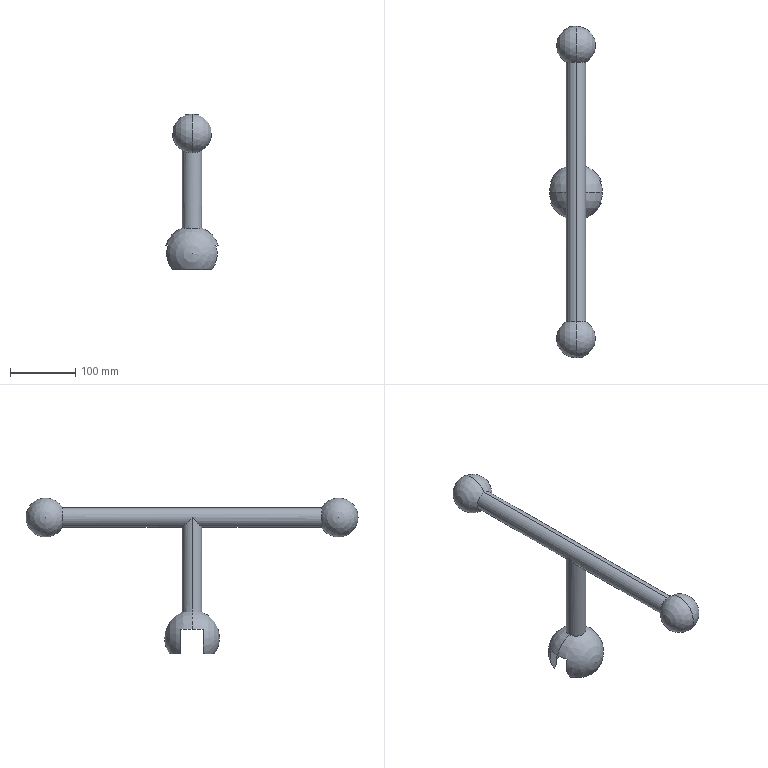Part | SolidWorks | features ICE 3, Chamfer 2, Revolution 2, Extrusion 1, MirrorPattern 1, RevCut 1 | 1 solid | 23 faces | box 80.921 x 510 x 239.694 mm | volume 716291 mm3 | sphere 8 | plane 7 | cylinder 6 | cone 2 | commonest cylinder face diameters 30 x4 60 x2
STEP:
#1=CARTESIAN_POINT('',(0.,-199.019,65.));
#2=VERTEX_POINT('',#1);
#3=CARTESIAN_POINT('',(0.,-199.019,95.));
#4=VERTEX_POINT('',#3);
#5=CARTESIAN_POINT('',(0.,-199.019,80.));
#6=DIRECTION('',(0.,-1.,0.));
#7=DIRECTION('',(0.,0.,-1.));
#8=AXIS2_PLACEMENT_3D('',#5,#6,#7);
#9=CIRCLE('',#8,15.);
#10=EDGE_CURVE('',#2,#4,#9,.T.);
#11=ORIENTED_EDGE('',*,*,#10,.T.);
#12=CARTESIAN_POINT('',(0.,-255.,80.));
#13=VERTEX_POINT('',#12);
#14=CARTESIAN_POINT('',(0.,-225.,80.));
#15=DIRECTION('',(1.,0.,0.));
#16=DIRECTION('',(0.,0.,-1.));
#17=AXIS2_PLACEMENT_3D('',#14,#15,#16);
#18=CIRCLE('',#17,30.);
#19=EDGE_CURVE('',#4,#13,#18,.T.);
#20=ORIENTED_EDGE('',*,*,#19,.T.);
#21=CARTESIAN_POINT('',(0.,-225.,80.));
#22=DIRECTION('',(-1.,0.,0.));
#23=DIRECTION('',(0.,0.,1.));
#24=AXIS2_PLACEMENT_3D('',#21,#22,#23);
#25=CIRCLE('',#24,30.);
#26=EDGE_CURVE('',#2,#13,#25,.T.);
#27=ORIENTED_EDGE('',*,*,#26,.F.);
#28=EDGE_LOOP('',(#11,#20,#27));
#29=FACE_OUTER_BOUND('',#28,.T.);
#30=CARTESIAN_POINT('',(0.,-225.,80.));
#31=DIRECTION('',(1.,0.,0.));
#32=DIRECTION('',(0.,0.,-1.));
#33=AXIS2_PLACEMENT_3D('',#30,#31,#32);
#34=SPHERICAL_SURFACE('',#33,30.);
#35=ADVANCED_FACE('',(#29),#34,.T.);
#36=CARTESIAN_POINT('',(0.,199.019,65.));
#37=VERTEX_POINT('',#36);
#38=CARTESIAN_POINT('',(0.,199.019,95.));
#39=VERTEX_POINT('',#38);
#40=CARTESIAN_POINT('',(0.,199.019,80.));
#41=DIRECTION('',(0.,1.,0.));
#42=DIRECTION('',(0.,0.,1.));
#43=AXIS2_PLACEMENT_3D('',#40,#41,#42);
#44=CIRCLE('',#43,15.);
#45=EDGE_CURVE('',#37,#39,#44,.T.);
#46=ORIENTED_EDGE('',*,*,#45,.T.);
#47=CARTESIAN_POINT('',(0.,255.,80.));
#48=VERTEX_POINT('',#47);
#49=CARTESIAN_POINT('',(0.,225.,80.));
#50=DIRECTION('',(-1.,0.,0.));
#51=DIRECTION('',(0.,0.,1.));
#52=AXIS2_PLACEMENT_3D('',#49,#50,#51);
#53=CIRCLE('',#52,30.);
#54=EDGE_CURVE('',#39,#48,#53,.T.);
#55=ORIENTED_EDGE('',*,*,#54,.T.);
#56=CARTESIAN_POINT('',(0.,225.,80.));
#57=DIRECTION('',(1.,0.,0.));
#58=DIRECTION('',(0.,0.,-1.));
#59=AXIS2_PLACEMENT_3D('',#56,#57,#58);
#60=CIRCLE('',#59,30.);
#61=EDGE_CURVE('',#37,#48,#60,.T.);
#62=ORIENTED_EDGE('',*,*,#61,.F.);
#63=EDGE_LOOP('',(#46,#55,#62));
#64=FACE_OUTER_BOUND('',#63,.T.);
#65=CARTESIAN_POINT('',(0.,225.,80.));
#66=DIRECTION('',(-1.,0.,0.));
#67=DIRECTION('',(0.,0.,-1.));
#68=AXIS2_PLACEMENT_3D('',#65,#66,#67);
#69=SPHERICAL_SURFACE('',#68,30.);
#70=ADVANCED_FACE('',(#64),#69,.T.);
#71=CARTESIAN_POINT('',(0.,0.,-75.));
#72=VERTEX_POINT('',#71);
#73=CARTESIAN_POINT('',(-21.424,0.,-84.));
#74=VERTEX_POINT('',#73);
#75=CARTESIAN_POINT('',(0.,0.,-105.));
#76=DIRECTION('',(0.,-1.,0.));
#77=DIRECTION('',(0.,0.,-1.));
#78=AXIS2_PLACEMENT_3D('',#75,#76,#77);
#79=CIRCLE('',#78,30.);
#80=EDGE_CURVE('',#72,#74,#79,.T.);
#81=ORIENTED_EDGE('',*,*,#80,.F.);
#82=CARTESIAN_POINT('',(21.424,0.,-84.));
#83=VERTEX_POINT('',#82);
#84=CARTESIAN_POINT('',(0.,0.,-105.));
#85=DIRECTION('',(0.,1.,0.));
#86=DIRECTION('',(-1.,0.,0.));
#87=AXIS2_PLACEMENT_3D('',#84,#85,#86);
#88=CIRCLE('',#87,30.);
#89=EDGE_CURVE('',#72,#83,#88,.T.);
#90=ORIENTED_EDGE('',*,*,#89,.T.);
#91=CARTESIAN_POINT('',(0.,0.,-84.));
#92=DIRECTION('',(0.,0.,-1.));
#93=DIRECTION('',(1.,0.,0.));
#94=AXIS2_PLACEMENT_3D('',#91,#92,#93);
#95=CIRCLE('',#94,21.424);
#96=EDGE_CURVE('',#83,#74,#95,.T.);
#97=ORIENTED_EDGE('',*,*,#96,.T.);
#98=EDGE_LOOP('',(#81,#90,#97));
#99=FACE_OUTER_BOUND('',#98,.T.);
#100=CARTESIAN_POINT('',(0.,0.,-105.));
#101=DIRECTION('',(0.,1.,0.));
#102=DIRECTION('',(-1.,0.,0.));
#103=AXIS2_PLACEMENT_3D('',#100,#101,#102);
#104=SPHERICAL_SURFACE('',#103,30.);
#105=ADVANCED_FACE('',(#99),#104,.F.);
#106=CARTESIAN_POINT('',(15.,0.,-65.235));
#107=VERTEX_POINT('',#106);
#108=CARTESIAN_POINT('',(-15.,0.,-65.235));
#109=VERTEX_POINT('',#108);
#110=CARTESIAN_POINT('',(0.,0.,-65.235));
#111=DIRECTION('',(0.,0.,-1.));
#112=DIRECTION('',(-1.,0.,0.));
#113=AXIS2_PLACEMENT_3D('',#110,#111,#112);
#114=CIRCLE('',#113,15.);
#115=EDGE_CURVE('',#107,#109,#114,.T.);
#116=ORIENTED_EDGE('',*,*,#115,.T.);
#117=CARTESIAN_POINT('',(-40.46,0.,-91.992));
#118=VERTEX_POINT('',#117);
#119=CARTESIAN_POINT('',(0.,0.,-105.));
#120=DIRECTION('',(0.,-1.,0.));
#121=DIRECTION('',(1.,0.,0.));
#122=AXIS2_PLACEMENT_3D('',#119,#120,#121);
#123=CIRCLE('',#122,42.5);
#124=EDGE_CURVE('',#109,#118,#123,.T.);
#125=ORIENTED_EDGE('',*,*,#124,.T.);
#126=CARTESIAN_POINT('',(-36.62,-17.204,-91.992));
#127=VERTEX_POINT('',#126);
#128=CARTESIAN_POINT('',(0.,0.,-91.992));
#129=DIRECTION('',(0.,0.,1.));
#130=DIRECTION('',(1.,0.,0.));
#131=AXIS2_PLACEMENT_3D('',#128,#129,#130);
#132=CIRCLE('',#131,40.46);
#133=EDGE_CURVE('',#118,#127,#132,.T.);
#134=ORIENTED_EDGE('',*,*,#133,.T.);
#135=CARTESIAN_POINT('',(-30.008,-17.204,-129.694));
#136=VERTEX_POINT('',#135);
#137=CARTESIAN_POINT('',(0.,-17.204,-105.));
#138=DIRECTION('',(0.,1.,0.));
#139=DIRECTION('',(0.,0.,1.));
#140=AXIS2_PLACEMENT_3D('',#137,#138,#139);
#141=CIRCLE('',#140,38.862);
#142=EDGE_CURVE('',#136,#127,#141,.T.);
#143=ORIENTED_EDGE('',*,*,#142,.F.);
#144=CARTESIAN_POINT('',(30.008,-17.204,-129.694));
#145=VERTEX_POINT('',#144);
#146=CARTESIAN_POINT('',(0.,0.,-129.694));
#147=DIRECTION('',(0.,0.,1.));
#148=DIRECTION('',(1.,0.,0.));
#149=AXIS2_PLACEMENT_3D('',#146,#147,#148);
#150=CIRCLE('',#149,34.59);
#151=EDGE_CURVE('',#136,#145,#150,.T.);
#152=ORIENTED_EDGE('',*,*,#151,.T.);
#153=CARTESIAN_POINT('',(36.62,-17.204,-91.992));
#154=VERTEX_POINT('',#153);
#155=CARTESIAN_POINT('',(0.,-17.204,-105.));
#156=DIRECTION('',(0.,1.,0.));
#157=DIRECTION('',(0.,0.,1.));
#158=AXIS2_PLACEMENT_3D('',#155,#156,#157);
#159=CIRCLE('',#158,38.862);
#160=EDGE_CURVE('',#154,#145,#159,.T.);
#161=ORIENTED_EDGE('',*,*,#160,.F.);
#162=CARTESIAN_POINT('',(40.46,0.,-91.992));
#163=VERTEX_POINT('',#162);
#164=CARTESIAN_POINT('',(0.,0.,-91.992));
#165=DIRECTION('',(0.,0.,1.));
#166=DIRECTION('',(1.,0.,0.));
#167=AXIS2_PLACEMENT_3D('',#164,#165,#166);
#168=CIRCLE('',#167,40.46);
#169=EDGE_CURVE('',#154,#163,#168,.T.);
#170=ORIENTED_EDGE('',*,*,#169,.T.);
#171=CARTESIAN_POINT('',(0.,0.,-105.));
#172=DIRECTION('',(0.,1.,0.));
#173=DIRECTION('',(0.,0.,1.));
#174=AXIS2_PLACEMENT_3D('',#171,#172,#173);
#175=CIRCLE('',#174,42.5);
#176=EDGE_CURVE('',#107,#163,#175,.T.);
#177=ORIENTED_EDGE('',*,*,#176,.F.);
#178=EDGE_LOOP('',(#116,#125,#134,#143,#152,#161,#170,#177));
#179=FACE_OUTER_BOUND('',#178,.T.);
#180=CARTESIAN_POINT('',(0.,0.,-105.));
#181=DIRECTION('',(0.,-1.,0.));
#182=DIRECTION('',(1.,0.,0.));
#183=AXIS2_PLACEMENT_3D('',#180,#181,#182);
#184=SPHERICAL_SURFACE('',#183,42.5);
#185=ADVANCED_FACE('',(#179),#184,.T.);
#186=CARTESIAN_POINT('',(-30.,0.,-84.));
#187=VERTEX_POINT('',#186);
#188=CARTESIAN_POINT('',(30.,0.,-84.));
#189=VERTEX_POINT('',#188);
#190=CARTESIAN_POINT('',(0.,0.,-84.));
#191=DIRECTION('',(0.,0.,1.));
#192=DIRECTION('',(1.,0.,0.));
#193=AXIS2_PLACEMENT_3D('',#190,#191,#192);
#194=CIRCLE('',#193,30.);
#195=EDGE_CURVE('',#187,#189,#194,.T.);
#196=ORIENTED_EDGE('',*,*,#195,.T.);
#197=CARTESIAN_POINT('',(30.,0.,-91.992));
#198=VERTEX_POINT('',#197);
#199=CARTESIAN_POINT('',(30.,0.,-84.));
#200=DIRECTION('',(0.,0.,-1.));
#201=VECTOR('',#200,1000.);
#202=LINE('',#199,#201);
#203=EDGE_CURVE('',#189,#198,#202,.T.);
#204=ORIENTED_EDGE('',*,*,#203,.T.);
#205=CARTESIAN_POINT('',(24.577,-17.204,-91.992));
#206=VERTEX_POINT('',#205);
#207=CARTESIAN_POINT('',(0.,0.,-91.992));
#208=DIRECTION('',(0.,0.,1.));
#209=DIRECTION('',(1.,0.,0.));
#210=AXIS2_PLACEMENT_3D('',#207,#208,#209);
#211=CIRCLE('',#210,30.);
#212=EDGE_CURVE('',#206,#198,#211,.T.);
#213=ORIENTED_EDGE('',*,*,#212,.F.);
#214=CARTESIAN_POINT('',(24.577,-17.204,-125.104));
#215=VERTEX_POINT('',#214);
#216=CARTESIAN_POINT('',(24.577,-17.204,-84.));
#217=DIRECTION('',(0.,0.,-1.));
#218=VECTOR('',#217,1000.);
#219=LINE('',#216,#218);
#220=EDGE_CURVE('',#206,#215,#219,.T.);
#221=ORIENTED_EDGE('',*,*,#220,.T.);
#222=CARTESIAN_POINT('',(-24.577,-17.204,-125.104));
#223=VERTEX_POINT('',#222);
#224=CARTESIAN_POINT('',(0.,0.,-125.104));
#225=DIRECTION('',(0.,0.,-1.));
#226=DIRECTION('',(1.,0.,0.));
#227=AXIS2_PLACEMENT_3D('',#224,#225,#226);
#228=CIRCLE('',#227,30.);
#229=EDGE_CURVE('',#215,#223,#228,.T.);
#230=ORIENTED_EDGE('',*,*,#229,.T.);
#231=CARTESIAN_POINT('',(-24.577,-17.204,-91.992));
#232=VERTEX_POINT('',#231);
#233=CARTESIAN_POINT('',(-24.577,-17.204,-84.));
#234=DIRECTION('',(0.,0.,1.));
#235=VECTOR('',#234,1000.);
#236=LINE('',#233,#235);
#237=EDGE_CURVE('',#223,#232,#236,.T.);
#238=ORIENTED_EDGE('',*,*,#237,.T.);
#239=CARTESIAN_POINT('',(-30.,0.,-91.992));
#240=VERTEX_POINT('',#239);
#241=CARTESIAN_POINT('',(0.,0.,-91.992));
#242=DIRECTION('',(0.,0.,1.));
#243=DIRECTION('',(1.,0.,0.));
#244=AXIS2_PLACEMENT_3D('',#241,#242,#243);
#245=CIRCLE('',#244,30.);
#246=EDGE_CURVE('',#240,#232,#245,.T.);
#247=ORIENTED_EDGE('',*,*,#246,.F.);
#248=CARTESIAN_POINT('',(-30.,0.,-84.));
#249=DIRECTION('',(0.,0.,-1.));
#250=VECTOR('',#249,1000.);
#251=LINE('',#248,#250);
#252=EDGE_CURVE('',#187,#240,#251,.T.);
#253=ORIENTED_EDGE('',*,*,#252,.F.);
#254=EDGE_LOOP('',(#196,#204,#213,#221,#230,#238,#247,#253));
#255=FACE_OUTER_BOUND('',#254,.T.);
#256=CARTESIAN_POINT('',(0.,0.,-84.));
#257=DIRECTION('',(0.,0.,-1.));
#258=DIRECTION('',(-1.,0.,0.));
#259=AXIS2_PLACEMENT_3D('',#256,#257,#258);
#260=CYLINDRICAL_SURFACE('',#259,30.);
#261=ADVANCED_FACE('',(#255),#260,.F.);
#262=CARTESIAN_POINT('',(15.,0.,80.));
#263=VERTEX_POINT('',#262);
#264=CARTESIAN_POINT('',(0.,15.,65.));
#265=VERTEX_POINT('',#264);
#266=CARTESIAN_POINT('',(15.,0.,80.));
#267=CARTESIAN_POINT('',(15.,8.787,71.213));
#268=CARTESIAN_POINT('',(8.787,15.,65.));
#269=CARTESIAN_POINT('',(0.,15.,65.));
#270=(BOUNDED_CURVE()B_SPLINE_CURVE(3,(#266,#267,#268,#269),.UNSPECIFIED.,.F.,.F.)B_SPLINE_CURVE_WITH_KNOTS((4,4),(4.712,6.283),.UNSPECIFIED.)CURVE()GEOMETRIC_REPRESENTATION_ITEM()RATIONAL_B_SPLINE_CURVE((1.,0.8047,0.8047,1.))REPRESENTATION_ITEM(''));
#271=EDGE_CURVE('',#263,#265,#270,.T.);
#272=ORIENTED_EDGE('',*,*,#271,.F.);
#273=CARTESIAN_POINT('',(15.,0.,80.));
#274=DIRECTION('',(0.,0.,-1.));
#275=VECTOR('',#274,1000.);
#276=LINE('',#273,#275);
#277=EDGE_CURVE('',#263,#107,#276,.T.);
#278=ORIENTED_EDGE('',*,*,#277,.T.);
#279=CARTESIAN_POINT('',(0.,0.,-65.235));
#280=DIRECTION('',(0.,0.,-1.));
#281=DIRECTION('',(-1.,0.,0.));
#282=AXIS2_PLACEMENT_3D('',#279,#280,#281);
#283=CIRCLE('',#282,15.);
#284=EDGE_CURVE('',#109,#107,#283,.T.);
#285=ORIENTED_EDGE('',*,*,#284,.F.);
#286=CARTESIAN_POINT('',(-15.,0.,80.));
#287=VERTEX_POINT('',#286);
#288=CARTESIAN_POINT('',(-15.,0.,80.));
#289=DIRECTION('',(0.,0.,-1.));
#290=VECTOR('',#289,1000.);
#291=LINE('',#288,#290);
#292=EDGE_CURVE('',#287,#109,#291,.T.);
#293=ORIENTED_EDGE('',*,*,#292,.F.);
#294=CARTESIAN_POINT('',(0.,15.,65.));
#295=CARTESIAN_POINT('',(-8.787,15.,65.));
#296=CARTESIAN_POINT('',(-15.,8.787,71.213));
#297=CARTESIAN_POINT('',(-15.,0.,80.));
#298=(BOUNDED_CURVE()B_SPLINE_CURVE(3,(#294,#295,#296,#297),.UNSPECIFIED.,.F.,.F.)B_SPLINE_CURVE_WITH_KNOTS((4,4),(0.,1.571),.UNSPECIFIED.)CURVE()GEOMETRIC_REPRESENTATION_ITEM()RATIONAL_B_SPLINE_CURVE((1.,0.8047,0.8047,1.))REPRESENTATION_ITEM(''));
#299=EDGE_CURVE('',#265,#287,#298,.T.);
#300=ORIENTED_EDGE('',*,*,#299,.F.);
#301=EDGE_LOOP('',(#272,#278,#285,#293,#300));
#302=FACE_OUTER_BOUND('',#301,.T.);
#303=CARTESIAN_POINT('',(0.,0.,80.));
#304=DIRECTION('',(0.,0.,-1.));
#305=DIRECTION('',(-1.,0.,0.));
#306=AXIS2_PLACEMENT_3D('',#303,#304,#305);
#307=CYLINDRICAL_SURFACE('',#306,15.);
#308=ADVANCED_FACE('',(#302),#307,.T.);
#309=CARTESIAN_POINT('',(0.,199.019,80.));
#310=DIRECTION('',(0.,1.,0.));
#311=DIRECTION('',(0.,0.,1.));
#312=AXIS2_PLACEMENT_3D('',#309,#310,#311);
#313=CIRCLE('',#312,15.);
#314=EDGE_CURVE('',#39,#37,#313,.T.);
#315=ORIENTED_EDGE('',*,*,#314,.F.);
#316=CARTESIAN_POINT('',(0.,200.,95.));
#317=DIRECTION('',(0.,-1.,0.));
#318=VECTOR('',#317,1000.);
#319=LINE('',#316,#318);
#320=EDGE_CURVE('',#39,#4,#319,.T.);
#321=ORIENTED_EDGE('',*,*,#320,.T.);
#322=ORIENTED_EDGE('',*,*,#10,.F.);
#323=CARTESIAN_POINT('',(0.,-15.,65.));
#324=VERTEX_POINT('',#323);
#325=CARTESIAN_POINT('',(0.,200.,65.));
#326=DIRECTION('',(0.,-1.,0.));
#327=VECTOR('',#326,1000.);
#328=LINE('',#325,#327);
#329=EDGE_CURVE('',#324,#2,#328,.T.);
#330=ORIENTED_EDGE('',*,*,#329,.F.);
#331=CARTESIAN_POINT('',(0.,-15.,65.));
#332=CARTESIAN_POINT('',(8.787,-15.,65.));
#333=CARTESIAN_POINT('',(15.,-8.787,71.213));
#334=CARTESIAN_POINT('',(15.,0.,80.));
#335=(BOUNDED_CURVE()B_SPLINE_CURVE(3,(#331,#332,#333,#334),.UNSPECIFIED.,.F.,.F.)B_SPLINE_CURVE_WITH_KNOTS((4,4),(0.,1.571),.UNSPECIFIED.)CURVE()GEOMETRIC_REPRESENTATION_ITEM()RATIONAL_B_SPLINE_CURVE((1.,0.8047,0.8047,1.))REPRESENTATION_ITEM(''));
#336=EDGE_CURVE('',#324,#263,#335,.T.);
#337=ORIENTED_EDGE('',*,*,#336,.T.);
#338=ORIENTED_EDGE('',*,*,#271,.T.);
#339=CARTESIAN_POINT('',(0.,200.,65.));
#340=DIRECTION('',(0.,-1.,0.));
#341=VECTOR('',#340,1000.);
#342=LINE('',#339,#341);
#343=EDGE_CURVE('',#37,#265,#342,.T.);
#344=ORIENTED_EDGE('',*,*,#343,.F.);
#345=EDGE_LOOP('',(#315,#321,#322,#330,#337,#338,#344));
#346=FACE_OUTER_BOUND('',#345,.T.);
#347=CARTESIAN_POINT('',(0.,200.,80.));
#348=DIRECTION('',(0.,-1.,0.));
#349=DIRECTION('',(0.,0.,-1.));
#350=AXIS2_PLACEMENT_3D('',#347,#348,#349);
#351=CYLINDRICAL_SURFACE('',#350,15.);
#352=ADVANCED_FACE('',(#346),#351,.T.);
#353=ORIENTED_EDGE('',*,*,#320,.F.);
#354=ORIENTED_EDGE('',*,*,#45,.F.);
#355=ORIENTED_EDGE('',*,*,#343,.T.);
#356=ORIENTED_EDGE('',*,*,#299,.T.);
#357=CARTESIAN_POINT('',(-15.,0.,80.));
#358=CARTESIAN_POINT('',(-15.,-8.787,71.213));
#359=CARTESIAN_POINT('',(-8.787,-15.,65.));
#360=CARTESIAN_POINT('',(0.,-15.,65.));
#361=(BOUNDED_CURVE()B_SPLINE_CURVE(3,(#357,#358,#359,#360),.UNSPECIFIED.,.F.,.F.)B_SPLINE_CURVE_WITH_KNOTS((4,4),(4.712,6.283),.UNSPECIFIED.)CURVE()GEOMETRIC_REPRESENTATION_ITEM()RATIONAL_B_SPLINE_CURVE((1.,0.8047,0.8047,1.))REPRESENTATION_ITEM(''));
#362=EDGE_CURVE('',#287,#324,#361,.T.);
#363=ORIENTED_EDGE('',*,*,#362,.T.);
#364=ORIENTED_EDGE('',*,*,#329,.T.);
#365=CARTESIAN_POINT('',(0.,-199.019,80.));
#366=DIRECTION('',(0.,-1.,0.));
#367=DIRECTION('',(0.,0.,-1.));
#368=AXIS2_PLACEMENT_3D('',#365,#366,#367);
#369=CIRCLE('',#368,15.);
#370=EDGE_CURVE('',#4,#2,#369,.T.);
#371=ORIENTED_EDGE('',*,*,#370,.F.);
#372=EDGE_LOOP('',(#353,#354,#355,#356,#363,#364,#371));
#373=FACE_OUTER_BOUND('',#372,.T.);
#374=CARTESIAN_POINT('',(0.,200.,80.));
#375=DIRECTION('',(0.,-1.,0.));
#376=DIRECTION('',(0.,0.,-1.));
#377=AXIS2_PLACEMENT_3D('',#374,#375,#376);
#378=CYLINDRICAL_SURFACE('',#377,15.);
#379=ADVANCED_FACE('',(#373),#378,.T.);
#380=ORIENTED_EDGE('',*,*,#277,.F.);
#381=ORIENTED_EDGE('',*,*,#336,.F.);
#382=ORIENTED_EDGE('',*,*,#362,.F.);
#383=ORIENTED_EDGE('',*,*,#292,.T.);
#384=ORIENTED_EDGE('',*,*,#115,.F.);
#385=EDGE_LOOP('',(#380,#381,#382,#383,#384));
#386=FACE_OUTER_BOUND('',#385,.T.);
#387=CARTESIAN_POINT('',(0.,0.,80.));
#388=DIRECTION('',(0.,0.,-1.));
#389=DIRECTION('',(-1.,0.,0.));
#390=AXIS2_PLACEMENT_3D('',#387,#388,#389);
#391=CYLINDRICAL_SURFACE('',#390,15.);
#392=ADVANCED_FACE('',(#386),#391,.T.);
#393=ORIENTED_EDGE('',*,*,#203,.F.);
#394=CARTESIAN_POINT('',(0.,0.,-84.));
#395=DIRECTION('',(0.,0.,1.));
#396=DIRECTION('',(1.,0.,0.));
#397=AXIS2_PLACEMENT_3D('',#394,#395,#396);
#398=CIRCLE('',#397,30.);
#399=EDGE_CURVE('',#189,#187,#398,.T.);
#400=ORIENTED_EDGE('',*,*,#399,.T.);
#401=ORIENTED_EDGE('',*,*,#252,.T.);
#402=CARTESIAN_POINT('',(-24.577,17.204,-91.992));
#403=VERTEX_POINT('',#402);
#404=CARTESIAN_POINT('',(0.,0.,-91.992));
#405=DIRECTION('',(0.,0.,1.));
#406=DIRECTION('',(1.,0.,0.));
#407=AXIS2_PLACEMENT_3D('',#404,#405,#406);
#408=CIRCLE('',#407,30.);
#409=EDGE_CURVE('',#403,#240,#408,.T.);
#410=ORIENTED_EDGE('',*,*,#409,.F.);
#411=CARTESIAN_POINT('',(-24.577,17.204,-125.104));
#412=VERTEX_POINT('',#411);
#413=CARTESIAN_POINT('',(-24.577,17.204,-84.));
#414=DIRECTION('',(0.,0.,1.));
#415=VECTOR('',#414,1000.);
#416=LINE('',#413,#415);
#417=EDGE_CURVE('',#412,#403,#416,.T.);
#418=ORIENTED_EDGE('',*,*,#417,.F.);
#419=CARTESIAN_POINT('',(24.577,17.204,-125.104));
#420=VERTEX_POINT('',#419);
#421=CARTESIAN_POINT('',(0.,0.,-125.104));
#422=DIRECTION('',(0.,0.,-1.));
#423=DIRECTION('',(1.,0.,0.));
#424=AXIS2_PLACEMENT_3D('',#421,#422,#423);
#425=CIRCLE('',#424,30.);
#426=EDGE_CURVE('',#412,#420,#425,.T.);
#427=ORIENTED_EDGE('',*,*,#426,.T.);
#428=CARTESIAN_POINT('',(24.577,17.204,-91.992));
#429=VERTEX_POINT('',#428);
#430=CARTESIAN_POINT('',(24.577,17.204,-84.));
#431=DIRECTION('',(0.,0.,-1.));
#432=VECTOR('',#431,1000.);
#433=LINE('',#430,#432);
#434=EDGE_CURVE('',#429,#420,#433,.T.);
#435=ORIENTED_EDGE('',*,*,#434,.F.);
#436=CARTESIAN_POINT('',(0.,0.,-91.992));
#437=DIRECTION('',(0.,0.,1.));
#438=DIRECTION('',(1.,0.,0.));
#439=AXIS2_PLACEMENT_3D('',#436,#437,#438);
#440=CIRCLE('',#439,30.);
#441=EDGE_CURVE('',#198,#429,#440,.T.);
#442=ORIENTED_EDGE('',*,*,#441,.F.);
#443=EDGE_LOOP('',(#393,#400,#401,#410,#418,#427,#435,#442));
#444=FACE_OUTER_BOUND('',#443,.T.);
#445=CARTESIAN_POINT('',(0.,0.,-84.));
#446=DIRECTION('',(0.,0.,-1.));
#447=DIRECTION('',(-1.,0.,0.));
#448=AXIS2_PLACEMENT_3D('',#445,#446,#447);
#449=CYLINDRICAL_SURFACE('',#448,30.);
#450=ADVANCED_FACE('',(#444),#449,.F.);
#451=ORIENTED_EDGE('',*,*,#124,.F.);
#452=ORIENTED_EDGE('',*,*,#284,.T.);
#453=ORIENTED_EDGE('',*,*,#176,.T.);
#454=CARTESIAN_POINT('',(36.62,17.204,-91.992));
#455=VERTEX_POINT('',#454);
#456=CARTESIAN_POINT('',(0.,0.,-91.992));
#457=DIRECTION('',(0.,0.,1.));
#458=DIRECTION('',(1.,0.,0.));
#459=AXIS2_PLACEMENT_3D('',#456,#457,#458);
#460=CIRCLE('',#459,40.46);
#461=EDGE_CURVE('',#163,#455,#460,.T.);
#462=ORIENTED_EDGE('',*,*,#461,.T.);
#463=CARTESIAN_POINT('',(30.008,17.204,-129.694));
#464=VERTEX_POINT('',#463);
#465=CARTESIAN_POINT('',(0.,17.204,-105.));
#466=DIRECTION('',(0.,1.,0.));
#467=DIRECTION('',(0.,0.,1.));
#468=AXIS2_PLACEMENT_3D('',#465,#466,#467);
#469=CIRCLE('',#468,38.862);
#470=EDGE_CURVE('',#455,#464,#469,.T.);
#471=ORIENTED_EDGE('',*,*,#470,.T.);
#472=CARTESIAN_POINT('',(-30.008,17.204,-129.694));
#473=VERTEX_POINT('',#472);
#474=CARTESIAN_POINT('',(0.,0.,-129.694));
#475=DIRECTION('',(0.,0.,1.));
#476=DIRECTION('',(1.,0.,0.));
#477=AXIS2_PLACEMENT_3D('',#474,#475,#476);
#478=CIRCLE('',#477,34.59);
#479=EDGE_CURVE('',#464,#473,#478,.T.);
#480=ORIENTED_EDGE('',*,*,#479,.T.);
#481=CARTESIAN_POINT('',(-36.62,17.204,-91.992));
#482=VERTEX_POINT('',#481);
#483=CARTESIAN_POINT('',(0.,17.204,-105.));
#484=DIRECTION('',(0.,1.,0.));
#485=DIRECTION('',(0.,0.,1.));
#486=AXIS2_PLACEMENT_3D('',#483,#484,#485);
#487=CIRCLE('',#486,38.862);
#488=EDGE_CURVE('',#473,#482,#487,.T.);
#489=ORIENTED_EDGE('',*,*,#488,.T.);
#490=CARTESIAN_POINT('',(0.,0.,-91.992));
#491=DIRECTION('',(0.,0.,1.));
#492=DIRECTION('',(1.,0.,0.));
#493=AXIS2_PLACEMENT_3D('',#490,#491,#492);
#494=CIRCLE('',#493,40.46);
#495=EDGE_CURVE('',#482,#118,#494,.T.);
#496=ORIENTED_EDGE('',*,*,#495,.T.);
#497=EDGE_LOOP('',(#451,#452,#453,#462,#471,#480,#489,#496));
#498=FACE_OUTER_BOUND('',#497,.T.);
#499=CARTESIAN_POINT('',(0.,0.,-105.));
#500=DIRECTION('',(0.,-1.,0.));
#501=DIRECTION('',(1.,0.,0.));
#502=AXIS2_PLACEMENT_3D('',#499,#500,#501);
#503=SPHERICAL_SURFACE('',#502,42.5);
#504=ADVANCED_FACE('',(#498),#503,.T.);
#505=ORIENTED_EDGE('',*,*,#89,.F.);
#506=ORIENTED_EDGE('',*,*,#80,.T.);
#507=CARTESIAN_POINT('',(0.,0.,-84.));
#508=DIRECTION('',(0.,0.,-1.));
#509=DIRECTION('',(1.,0.,0.));
#510=AXIS2_PLACEMENT_3D('',#507,#508,#509);
#511=CIRCLE('',#510,21.424);
#512=EDGE_CURVE('',#74,#83,#511,.T.);
#513=ORIENTED_EDGE('',*,*,#512,.T.);
#514=EDGE_LOOP('',(#505,#506,#513));
#515=FACE_OUTER_BOUND('',#514,.T.);
#516=CARTESIAN_POINT('',(0.,0.,-105.));
#517=DIRECTION('',(0.,1.,0.));
#518=DIRECTION('',(-1.,0.,0.));
#519=AXIS2_PLACEMENT_3D('',#516,#517,#518);
#520=SPHERICAL_SURFACE('',#519,30.);
#521=ADVANCED_FACE('',(#515),#520,.F.);
#522=ORIENTED_EDGE('',*,*,#195,.F.);
#523=ORIENTED_EDGE('',*,*,#399,.F.);
#524=EDGE_LOOP('',(#522,#523));
#525=FACE_OUTER_BOUND('',#524,.T.);
#526=ORIENTED_EDGE('',*,*,#512,.F.);
#527=ORIENTED_EDGE('',*,*,#96,.F.);
#528=EDGE_LOOP('',(#526,#527));
#529=FACE_BOUND('',#528,.T.);
#530=CARTESIAN_POINT('',(0.,0.,-84.));
#531=DIRECTION('',(0.,0.,1.));
#532=DIRECTION('',(1.,0.,0.));
#533=AXIS2_PLACEMENT_3D('',#530,#531,#532);
#534=PLANE('',#533);
#535=ADVANCED_FACE('',(#525,#529),#534,.F.);
#536=ORIENTED_EDGE('',*,*,#488,.F.);
#537=CARTESIAN_POINT('',(-30.008,17.204,-129.694));
#538=CARTESIAN_POINT('',(-28.217,17.204,-128.14));
#539=CARTESIAN_POINT('',(-26.411,17.204,-126.606));
#540=CARTESIAN_POINT('',(-24.577,17.204,-125.104));
#541=B_SPLINE_CURVE_WITH_KNOTS('',3,(#537,#538,#539,#540),.UNSPECIFIED.,.F.,.F.,(4,4),(0.,0.007111),.UNSPECIFIED.);
#542=EDGE_CURVE('',#473,#412,#541,.T.);
#543=ORIENTED_EDGE('',*,*,#542,.T.);
#544=ORIENTED_EDGE('',*,*,#417,.T.);
#545=CARTESIAN_POINT('',(-75.5,17.204,-91.992));
#546=DIRECTION('',(1.,0.,0.));
#547=VECTOR('',#546,1000.);
#548=LINE('',#545,#547);
#549=EDGE_CURVE('',#482,#403,#548,.T.);
#550=ORIENTED_EDGE('',*,*,#549,.F.);
#551=EDGE_LOOP('',(#536,#543,#544,#550));
#552=FACE_OUTER_BOUND('',#551,.T.);
#553=CARTESIAN_POINT('',(-75.5,17.204,-178.216));
#554=DIRECTION('',(0.,1.,0.));
#555=DIRECTION('',(0.,0.,1.));
#556=AXIS2_PLACEMENT_3D('',#553,#554,#555);
#557=PLANE('',#556);
#558=ADVANCED_FACE('',(#552),#557,.F.);
#559=ORIENTED_EDGE('',*,*,#409,.T.);
#560=ORIENTED_EDGE('',*,*,#246,.T.);
#561=CARTESIAN_POINT('',(-75.5,-17.204,-91.992));
#562=DIRECTION('',(1.,0.,0.));
#563=VECTOR('',#562,1000.);
#564=LINE('',#561,#563);
#565=EDGE_CURVE('',#127,#232,#564,.T.);
#566=ORIENTED_EDGE('',*,*,#565,.F.);
#567=ORIENTED_EDGE('',*,*,#133,.F.);
#568=ORIENTED_EDGE('',*,*,#495,.F.);
#569=ORIENTED_EDGE('',*,*,#549,.T.);
#570=EDGE_LOOP('',(#559,#560,#566,#567,#568,#569));
#571=FACE_OUTER_BOUND('',#570,.T.);
#572=CARTESIAN_POINT('',(-75.5,17.204,-91.992));
#573=DIRECTION('',(0.,0.,1.));
#574=DIRECTION('',(1.,0.,0.));
#575=AXIS2_PLACEMENT_3D('',#572,#573,#574);
#576=PLANE('',#575);
#577=ADVANCED_FACE('',(#571),#576,.F.);
#578=ORIENTED_EDGE('',*,*,#237,.F.);
#579=CARTESIAN_POINT('',(-24.577,-17.204,-125.104));
#580=CARTESIAN_POINT('',(-26.411,-17.204,-126.606));
#581=CARTESIAN_POINT('',(-28.217,-17.204,-128.14));
#582=CARTESIAN_POINT('',(-30.008,-17.204,-129.694));
#583=B_SPLINE_CURVE_WITH_KNOTS('',3,(#579,#580,#581,#582),.UNSPECIFIED.,.F.,.F.,(4,4),(0.,0.007111),.UNSPECIFIED.);
#584=EDGE_CURVE('',#223,#136,#583,.T.);
#585=ORIENTED_EDGE('',*,*,#584,.T.);
#586=ORIENTED_EDGE('',*,*,#142,.T.);
#587=ORIENTED_EDGE('',*,*,#565,.T.);
#588=EDGE_LOOP('',(#578,#585,#586,#587));
#589=FACE_OUTER_BOUND('',#588,.T.);
#590=CARTESIAN_POINT('',(-75.5,-17.204,-178.216));
#591=DIRECTION('',(0.,1.,0.));
#592=DIRECTION('',(0.,0.,1.));
#593=AXIS2_PLACEMENT_3D('',#590,#591,#592);
#594=PLANE('',#593);
#595=ADVANCED_FACE('',(#589),#594,.T.);
#596=ORIENTED_EDGE('',*,*,#160,.T.);
#597=CARTESIAN_POINT('',(30.008,-17.204,-129.694));
#598=CARTESIAN_POINT('',(28.217,-17.204,-128.14));
#599=CARTESIAN_POINT('',(26.411,-17.204,-126.606));
#600=CARTESIAN_POINT('',(24.577,-17.204,-125.104));
#601=B_SPLINE_CURVE_WITH_KNOTS('',3,(#597,#598,#599,#600),.UNSPECIFIED.,.F.,.F.,(4,4),(0.,0.007111),.UNSPECIFIED.);
#602=EDGE_CURVE('',#145,#215,#601,.T.);
#603=ORIENTED_EDGE('',*,*,#602,.T.);
#604=ORIENTED_EDGE('',*,*,#220,.F.);
#605=CARTESIAN_POINT('',(-75.5,-17.204,-91.992));
#606=DIRECTION('',(1.,0.,0.));
#607=VECTOR('',#606,1000.);
#608=LINE('',#605,#607);
#609=EDGE_CURVE('',#206,#154,#608,.T.);
#610=ORIENTED_EDGE('',*,*,#609,.T.);
#611=EDGE_LOOP('',(#596,#603,#604,#610));
#612=FACE_OUTER_BOUND('',#611,.T.);
#613=CARTESIAN_POINT('',(-75.5,-17.204,-178.216));
#614=DIRECTION('',(0.,1.,0.));
#615=DIRECTION('',(0.,0.,1.));
#616=AXIS2_PLACEMENT_3D('',#613,#614,#615);
#617=PLANE('',#616);
#618=ADVANCED_FACE('',(#612),#617,.T.);
#619=ORIENTED_EDGE('',*,*,#212,.T.);
#620=ORIENTED_EDGE('',*,*,#441,.T.);
#621=CARTESIAN_POINT('',(-75.5,17.204,-91.992));
#622=DIRECTION('',(1.,0.,0.));
#623=VECTOR('',#622,1000.);
#624=LINE('',#621,#623);
#625=EDGE_CURVE('',#429,#455,#624,.T.);
#626=ORIENTED_EDGE('',*,*,#625,.T.);
#627=ORIENTED_EDGE('',*,*,#461,.F.);
#628=ORIENTED_EDGE('',*,*,#169,.F.);
#629=ORIENTED_EDGE('',*,*,#609,.F.);
#630=EDGE_LOOP('',(#619,#620,#626,#627,#628,#629));
#631=FACE_OUTER_BOUND('',#630,.T.);
#632=CARTESIAN_POINT('',(-75.5,17.204,-91.992));
#633=DIRECTION('',(0.,0.,1.));
#634=DIRECTION('',(1.,0.,0.));
#635=AXIS2_PLACEMENT_3D('',#632,#633,#634);
#636=PLANE('',#635);
#637=ADVANCED_FACE('',(#631),#636,.F.);
#638=ORIENTED_EDGE('',*,*,#434,.T.);
#639=CARTESIAN_POINT('',(24.577,17.204,-125.104));
#640=CARTESIAN_POINT('',(26.411,17.204,-126.606));
#641=CARTESIAN_POINT('',(28.217,17.204,-128.14));
#642=CARTESIAN_POINT('',(30.008,17.204,-129.694));
#643=B_SPLINE_CURVE_WITH_KNOTS('',3,(#639,#640,#641,#642),.UNSPECIFIED.,.F.,.F.,(4,4),(0.,0.007111),.UNSPECIFIED.);
#644=EDGE_CURVE('',#420,#464,#643,.T.);
#645=ORIENTED_EDGE('',*,*,#644,.T.);
#646=ORIENTED_EDGE('',*,*,#470,.F.);
#647=ORIENTED_EDGE('',*,*,#625,.F.);
#648=EDGE_LOOP('',(#638,#645,#646,#647));
#649=FACE_OUTER_BOUND('',#648,.T.);
#650=CARTESIAN_POINT('',(-75.5,17.204,-178.216));
#651=DIRECTION('',(0.,1.,0.));
#652=DIRECTION('',(0.,0.,1.));
#653=AXIS2_PLACEMENT_3D('',#650,#651,#652);
#654=PLANE('',#653);
#655=ADVANCED_FACE('',(#649),#654,.F.);
#656=ORIENTED_EDGE('',*,*,#602,.F.);
#657=ORIENTED_EDGE('',*,*,#151,.F.);
#658=ORIENTED_EDGE('',*,*,#584,.F.);
#659=ORIENTED_EDGE('',*,*,#229,.F.);
#660=EDGE_LOOP('',(#656,#657,#658,#659));
#661=FACE_OUTER_BOUND('',#660,.T.);
#662=CARTESIAN_POINT('',(0.,0.,-125.104));
#663=DIRECTION('',(0.,0.,-1.));
#664=DIRECTION('',(-1.,0.,0.));
#665=AXIS2_PLACEMENT_3D('',#662,#663,#664);
#666=CONICAL_SURFACE('',#665,30.,0.7854);
#667=ADVANCED_FACE('',(#661),#666,.F.);
#668=ORIENTED_EDGE('',*,*,#542,.F.);
#669=ORIENTED_EDGE('',*,*,#479,.F.);
#670=ORIENTED_EDGE('',*,*,#644,.F.);
#671=ORIENTED_EDGE('',*,*,#426,.F.);
#672=EDGE_LOOP('',(#668,#669,#670,#671));
#673=FACE_OUTER_BOUND('',#672,.T.);
#674=CARTESIAN_POINT('',(0.,0.,-125.104));
#675=DIRECTION('',(0.,0.,-1.));
#676=DIRECTION('',(-1.,0.,0.));
#677=AXIS2_PLACEMENT_3D('',#674,#675,#676);
#678=CONICAL_SURFACE('',#677,30.,0.7854);
#679=ADVANCED_FACE('',(#673),#678,.F.);
#680=ORIENTED_EDGE('',*,*,#54,.F.);
#681=ORIENTED_EDGE('',*,*,#314,.T.);
#682=ORIENTED_EDGE('',*,*,#61,.T.);
#683=EDGE_LOOP('',(#680,#681,#682));
#684=FACE_OUTER_BOUND('',#683,.T.);
#685=CARTESIAN_POINT('',(0.,225.,80.));
#686=DIRECTION('',(-1.,0.,0.));
#687=DIRECTION('',(0.,0.,-1.));
#688=AXIS2_PLACEMENT_3D('',#685,#686,#687);
#689=SPHERICAL_SURFACE('',#688,30.);
#690=ADVANCED_FACE('',(#684),#689,.T.);
#691=ORIENTED_EDGE('',*,*,#19,.F.);
#692=ORIENTED_EDGE('',*,*,#370,.T.);
#693=ORIENTED_EDGE('',*,*,#26,.T.);
#694=EDGE_LOOP('',(#691,#692,#693));
#695=FACE_OUTER_BOUND('',#694,.T.);
#696=CARTESIAN_POINT('',(0.,-225.,80.));
#697=DIRECTION('',(1.,0.,0.));
#698=DIRECTION('',(0.,0.,-1.));
#699=AXIS2_PLACEMENT_3D('',#696,#697,#698);
#700=SPHERICAL_SURFACE('',#699,30.);
#701=ADVANCED_FACE('',(#695),#700,.T.);
#702=CLOSED_SHELL('',(#35,#70,#105,#185,#261,#308,#352,#379,#392,#450,#504,#521,#535,#558,#577,#595,#618,#637,#655,#667,#679,#690,#701));
#703=MANIFOLD_SOLID_BREP('',#702);
#704=CARTESIAN_POINT('',(0.,0.,0.));
#705=DIRECTION('',(0.,0.,1.));
#706=DIRECTION('',(1.,0.,0.));
#707=AXIS2_PLACEMENT_3D('',#704,#705,#706);
#708=(LENGTH_UNIT()NAMED_UNIT(*)SI_UNIT(.MILLI.,.METRE.));
#709=UNCERTAINTY_MEASURE_WITH_UNIT(LENGTH_MEASURE(0.00001),#708,'','');
#710=(NAMED_UNIT(*)PLANE_ANGLE_UNIT()SI_UNIT($,.RADIAN.));
#711=(NAMED_UNIT(*)SI_UNIT($,.STERADIAN.)SOLID_ANGLE_UNIT());
#712=(GEOMETRIC_REPRESENTATION_CONTEXT(3)GLOBAL_UNCERTAINTY_ASSIGNED_CONTEXT((#709))GLOBAL_UNIT_ASSIGNED_CONTEXT((#708,#710,#711))REPRESENTATION_CONTEXT('',''));
#713=ADVANCED_BREP_SHAPE_REPRESENTATION('',(#703,#707),#712);